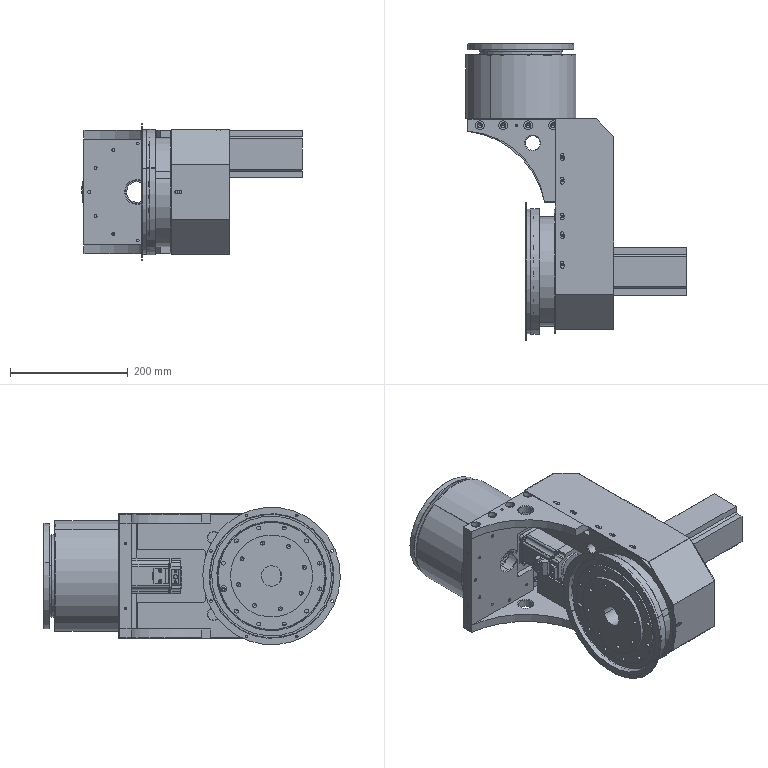Part | SolidWorks | features InContextFeatHolder 28, CompositeCurve 7 | 30 solids | 1866 faces | box 375 x 504.5 x 234 mm | volume 8003020 mm3 | cylinder 1092 | plane 473 | cone 277 | torus 22 | sphere 2 | commonest cylinder face diameters 5 x132 12.5 x108 6.6 x102 6.8 x72 11 x50 28.123 x50